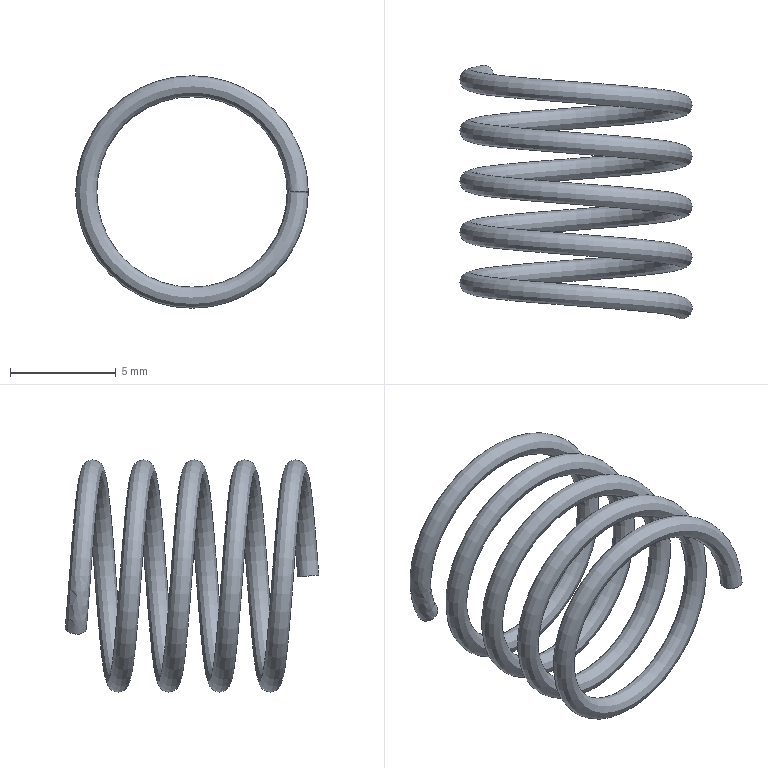Part | NX | features BREP 1 | 1 solid | 3 faces | box 11 x 11.998 x 11 mm | volume 113.166 mm3 | plane 2 | spline 1
STEP:
#1=CARTESIAN_POINT('',(5.,-0.4985,0.03809));
#2=VERTEX_POINT('',#1);
#3=CARTESIAN_POINT('',(5.,0.,0.));
#4=DIRECTION('',(0.,0.07617,0.9971));
#5=DIRECTION('',(0.,-0.9971,0.07617));
#6=AXIS2_PLACEMENT_3D('',#3,#4,#5);
#7=CIRCLE('',#6,0.5);
#8=EDGE_CURVE('',#2,#2,#7,.T.);
#9=ORIENTED_EDGE('',*,*,#8,.F.);
#10=EDGE_LOOP('',(#9));
#11=FACE_BOUND('',#10,.T.);
#12=CARTESIAN_POINT('',(5.,0.4985,-0.03809));
#13=DIRECTION('',(0.,-0.07617,-0.9971));
#14=DIRECTION('',(0.,-0.9971,0.07617));
#15=AXIS2_PLACEMENT_3D('',#12,#13,#14);
#16=PLANE('',#15);
#17=ADVANCED_FACE('',(#11),#16,.T.);
#18=CARTESIAN_POINT('',(-4.311,10.502,-2.533));
#19=VERTEX_POINT('',#18);
#20=CARTESIAN_POINT('',(-4.33,11.001,-2.5));
#21=DIRECTION('',(-0.4985,-0.07617,0.8635));
#22=DIRECTION('',(0.866,0.,0.5));
#23=AXIS2_PLACEMENT_3D('',#20,#21,#22);
#24=CIRCLE('',#23,0.5);
#25=EDGE_CURVE('',#19,#19,#24,.T.);
#26=ORIENTED_EDGE('',*,*,#25,.F.);
#27=EDGE_LOOP('',(#26));
#28=FACE_BOUND('',#27,.T.);
#29=CARTESIAN_POINT('',(-4.349,11.499,-2.467));
#30=DIRECTION('',(-0.4985,-0.07617,0.8635));
#31=DIRECTION('',(-0.866,0.,-0.5));
#32=AXIS2_PLACEMENT_3D('',#29,#30,#31);
#33=PLANE('',#32);
#34=ADVANCED_FACE('',(#28),#33,.F.);
#35=ORIENTED_EDGE('',*,*,#8,.T.);
#36=EDGE_LOOP('',(#35));
#37=FACE_BOUND('',#36,.T.);
#38=ORIENTED_EDGE('',*,*,#25,.T.);
#39=EDGE_LOOP('',(#38));
#40=FACE_BOUND('',#39,.T.);
#41=CARTESIAN_POINT('',(5.,-0.4985,0.03809));
#42=CARTESIAN_POINT('',(4.988,-0.3785,1.663));
#43=CARTESIAN_POINT('',(4.023,-0.2585,2.97));
#44=CARTESIAN_POINT('',(3.058,-0.1385,4.277));
#45=CARTESIAN_POINT('',(1.509,-0.01855,4.767));
#46=CARTESIAN_POINT('',(-0.04005,0.1015,5.257));
#47=CARTESIAN_POINT('',(-1.581,0.2215,4.744));
#48=CARTESIAN_POINT('',(-3.123,0.3415,4.23));
#49=CARTESIAN_POINT('',(-4.067,0.4615,2.908));
#50=CARTESIAN_POINT('',(-5.012,0.5815,1.587));
#51=CARTESIAN_POINT('',(-5.,0.7015,-0.03809));
#52=CARTESIAN_POINT('',(-4.988,0.8215,-1.663));
#53=CARTESIAN_POINT('',(-4.023,0.9415,-2.97));
#54=CARTESIAN_POINT('',(-3.058,1.061,-4.277));
#55=CARTESIAN_POINT('',(-1.509,1.181,-4.767));
#56=CARTESIAN_POINT('',(0.04005,1.301,-5.257));
#57=CARTESIAN_POINT('',(1.581,1.421,-4.744));
#58=CARTESIAN_POINT('',(3.123,1.541,-4.23));
#59=CARTESIAN_POINT('',(4.067,1.661,-2.908));
#60=CARTESIAN_POINT('',(5.012,1.781,-1.587));
#61=CARTESIAN_POINT('',(5.,1.901,0.03809));
#62=CARTESIAN_POINT('',(4.988,2.021,1.663));
#63=CARTESIAN_POINT('',(4.023,2.141,2.97));
#64=CARTESIAN_POINT('',(3.058,2.261,4.277));
#65=CARTESIAN_POINT('',(1.509,2.381,4.767));
#66=CARTESIAN_POINT('',(-0.04005,2.501,5.257));
#67=CARTESIAN_POINT('',(-1.581,2.621,4.744));
#68=CARTESIAN_POINT('',(-3.123,2.741,4.23));
#69=CARTESIAN_POINT('',(-4.067,2.861,2.908));
#70=CARTESIAN_POINT('',(-5.012,2.981,1.587));
#71=CARTESIAN_POINT('',(-5.,3.101,-0.03809));
#72=CARTESIAN_POINT('',(-4.988,3.221,-1.663));
#73=CARTESIAN_POINT('',(-4.023,3.341,-2.97));
#74=CARTESIAN_POINT('',(-3.058,3.461,-4.277));
#75=CARTESIAN_POINT('',(-1.509,3.581,-4.767));
#76=CARTESIAN_POINT('',(0.04005,3.701,-5.257));
#77=CARTESIAN_POINT('',(1.581,3.821,-4.744));
#78=CARTESIAN_POINT('',(3.123,3.941,-4.23));
#79=CARTESIAN_POINT('',(4.067,4.061,-2.908));
#80=CARTESIAN_POINT('',(5.012,4.181,-1.587));
#81=CARTESIAN_POINT('',(5.,4.301,0.03809));
#82=CARTESIAN_POINT('',(4.988,4.421,1.663));
#83=CARTESIAN_POINT('',(4.023,4.541,2.97));
#84=CARTESIAN_POINT('',(3.058,4.661,4.277));
#85=CARTESIAN_POINT('',(1.509,4.781,4.767));
#86=CARTESIAN_POINT('',(-0.04005,4.901,5.257));
#87=CARTESIAN_POINT('',(-1.581,5.021,4.744));
#88=CARTESIAN_POINT('',(-3.123,5.141,4.23));
#89=CARTESIAN_POINT('',(-4.067,5.261,2.908));
#90=CARTESIAN_POINT('',(-5.012,5.381,1.587));
#91=CARTESIAN_POINT('',(-5.,5.501,-0.03809));
#92=CARTESIAN_POINT('',(-4.988,5.621,-1.663));
#93=CARTESIAN_POINT('',(-4.023,5.741,-2.97));
#94=CARTESIAN_POINT('',(-3.058,5.861,-4.277));
#95=CARTESIAN_POINT('',(-1.509,5.981,-4.767));
#96=CARTESIAN_POINT('',(0.04005,6.101,-5.257));
#97=CARTESIAN_POINT('',(1.581,6.221,-4.744));
#98=CARTESIAN_POINT('',(3.123,6.341,-4.23));
#99=CARTESIAN_POINT('',(4.067,6.461,-2.908));
#100=CARTESIAN_POINT('',(5.012,6.581,-1.587));
#101=CARTESIAN_POINT('',(5.,6.701,0.03809));
#102=CARTESIAN_POINT('',(4.988,6.821,1.663));
#103=CARTESIAN_POINT('',(4.023,6.941,2.97));
#104=CARTESIAN_POINT('',(3.058,7.061,4.277));
#105=CARTESIAN_POINT('',(1.509,7.181,4.767));
#106=CARTESIAN_POINT('',(-0.04005,7.301,5.257));
#107=CARTESIAN_POINT('',(-1.581,7.421,4.744));
#108=CARTESIAN_POINT('',(-3.123,7.541,4.23));
#109=CARTESIAN_POINT('',(-4.067,7.661,2.908));
#110=CARTESIAN_POINT('',(-5.012,7.781,1.587));
#111=CARTESIAN_POINT('',(-5.,7.901,-0.03809));
#112=CARTESIAN_POINT('',(-4.988,8.021,-1.663));
#113=CARTESIAN_POINT('',(-4.023,8.141,-2.97));
#114=CARTESIAN_POINT('',(-3.058,8.261,-4.277));
#115=CARTESIAN_POINT('',(-1.509,8.381,-4.767));
#116=CARTESIAN_POINT('',(0.04005,8.501,-5.257));
#117=CARTESIAN_POINT('',(1.581,8.621,-4.744));
#118=CARTESIAN_POINT('',(3.123,8.741,-4.23));
#119=CARTESIAN_POINT('',(4.067,8.861,-2.908));
#120=CARTESIAN_POINT('',(5.012,8.981,-1.587));
#121=CARTESIAN_POINT('',(5.,9.101,0.03809));
#122=CARTESIAN_POINT('',(4.988,9.221,1.663));
#123=CARTESIAN_POINT('',(4.023,9.341,2.97));
#124=CARTESIAN_POINT('',(3.058,9.461,4.277));
#125=CARTESIAN_POINT('',(1.509,9.581,4.767));
#126=CARTESIAN_POINT('',(-0.04005,9.701,5.257));
#127=CARTESIAN_POINT('',(-1.581,9.821,4.744));
#128=CARTESIAN_POINT('',(-3.123,9.941,4.23));
#129=CARTESIAN_POINT('',(-4.067,10.061,2.908));
#130=CARTESIAN_POINT('',(-5.012,10.181,1.587));
#131=CARTESIAN_POINT('',(-5.,10.301,-0.03809));
#132=CARTESIAN_POINT('',(-4.99,10.4,-1.378));
#133=CARTESIAN_POINT('',(-4.311,10.502,-2.533));
#134=CARTESIAN_POINT('',(6.,-0.4985,0.03809));
#135=CARTESIAN_POINT('',(5.988,-0.3785,1.988));
#136=CARTESIAN_POINT('',(4.832,-0.2585,3.558));
#137=CARTESIAN_POINT('',(3.676,-0.1385,5.127));
#138=CARTESIAN_POINT('',(1.818,-0.01855,5.718));
#139=CARTESIAN_POINT('',(-0.04005,0.1015,6.309));
#140=CARTESIAN_POINT('',(-1.89,0.2215,5.695));
#141=CARTESIAN_POINT('',(-3.741,0.3415,5.08));
#142=CARTESIAN_POINT('',(-4.876,0.4615,3.496));
#143=CARTESIAN_POINT('',(-6.012,0.5815,1.911));
#144=CARTESIAN_POINT('',(-6.,0.7015,-0.03809));
#145=CARTESIAN_POINT('',(-5.988,0.8215,-1.988));
#146=CARTESIAN_POINT('',(-4.832,0.9415,-3.558));
#147=CARTESIAN_POINT('',(-3.676,1.061,-5.127));
#148=CARTESIAN_POINT('',(-1.818,1.181,-5.718));
#149=CARTESIAN_POINT('',(0.04005,1.301,-6.309));
#150=CARTESIAN_POINT('',(1.89,1.421,-5.695));
#151=CARTESIAN_POINT('',(3.741,1.541,-5.08));
#152=CARTESIAN_POINT('',(4.876,1.661,-3.496));
#153=CARTESIAN_POINT('',(6.012,1.781,-1.911));
#154=CARTESIAN_POINT('',(6.,1.901,0.03809));
#155=CARTESIAN_POINT('',(5.988,2.021,1.988));
#156=CARTESIAN_POINT('',(4.832,2.141,3.558));
#157=CARTESIAN_POINT('',(3.676,2.261,5.127));
#158=CARTESIAN_POINT('',(1.818,2.381,5.718));
#159=CARTESIAN_POINT('',(-0.04005,2.501,6.309));
#160=CARTESIAN_POINT('',(-1.89,2.621,5.695));
#161=CARTESIAN_POINT('',(-3.741,2.741,5.08));
#162=CARTESIAN_POINT('',(-4.876,2.861,3.496));
#163=CARTESIAN_POINT('',(-6.012,2.981,1.911));
#164=CARTESIAN_POINT('',(-6.,3.101,-0.03809));
#165=CARTESIAN_POINT('',(-5.988,3.221,-1.988));
#166=CARTESIAN_POINT('',(-4.832,3.341,-3.558));
#167=CARTESIAN_POINT('',(-3.676,3.461,-5.127));
#168=CARTESIAN_POINT('',(-1.818,3.581,-5.718));
#169=CARTESIAN_POINT('',(0.04005,3.701,-6.309));
#170=CARTESIAN_POINT('',(1.89,3.821,-5.695));
#171=CARTESIAN_POINT('',(3.741,3.941,-5.08));
#172=CARTESIAN_POINT('',(4.876,4.061,-3.496));
#173=CARTESIAN_POINT('',(6.012,4.181,-1.911));
#174=CARTESIAN_POINT('',(6.,4.301,0.03809));
#175=CARTESIAN_POINT('',(5.988,4.421,1.988));
#176=CARTESIAN_POINT('',(4.832,4.541,3.558));
#177=CARTESIAN_POINT('',(3.676,4.661,5.127));
#178=CARTESIAN_POINT('',(1.818,4.781,5.718));
#179=CARTESIAN_POINT('',(-0.04005,4.901,6.309));
#180=CARTESIAN_POINT('',(-1.89,5.021,5.695));
#181=CARTESIAN_POINT('',(-3.741,5.141,5.08));
#182=CARTESIAN_POINT('',(-4.876,5.261,3.496));
#183=CARTESIAN_POINT('',(-6.012,5.381,1.911));
#184=CARTESIAN_POINT('',(-6.,5.501,-0.03809));
#185=CARTESIAN_POINT('',(-5.988,5.621,-1.988));
#186=CARTESIAN_POINT('',(-4.832,5.741,-3.558));
#187=CARTESIAN_POINT('',(-3.676,5.861,-5.127));
#188=CARTESIAN_POINT('',(-1.818,5.981,-5.718));
#189=CARTESIAN_POINT('',(0.04005,6.101,-6.309));
#190=CARTESIAN_POINT('',(1.89,6.221,-5.695));
#191=CARTESIAN_POINT('',(3.741,6.341,-5.08));
#192=CARTESIAN_POINT('',(4.876,6.461,-3.496));
#193=CARTESIAN_POINT('',(6.012,6.581,-1.911));
#194=CARTESIAN_POINT('',(6.,6.701,0.03809));
#195=CARTESIAN_POINT('',(5.988,6.821,1.988));
#196=CARTESIAN_POINT('',(4.832,6.941,3.558));
#197=CARTESIAN_POINT('',(3.676,7.061,5.127));
#198=CARTESIAN_POINT('',(1.818,7.181,5.718));
#199=CARTESIAN_POINT('',(-0.04005,7.301,6.309));
#200=CARTESIAN_POINT('',(-1.89,7.421,5.695));
#201=CARTESIAN_POINT('',(-3.741,7.541,5.08));
#202=CARTESIAN_POINT('',(-4.876,7.661,3.496));
#203=CARTESIAN_POINT('',(-6.012,7.781,1.911));
#204=CARTESIAN_POINT('',(-6.,7.901,-0.03809));
#205=CARTESIAN_POINT('',(-5.988,8.021,-1.988));
#206=CARTESIAN_POINT('',(-4.832,8.141,-3.558));
#207=CARTESIAN_POINT('',(-3.676,8.261,-5.127));
#208=CARTESIAN_POINT('',(-1.818,8.381,-5.718));
#209=CARTESIAN_POINT('',(0.04005,8.501,-6.309));
#210=CARTESIAN_POINT('',(1.89,8.621,-5.695));
#211=CARTESIAN_POINT('',(3.741,8.741,-5.08));
#212=CARTESIAN_POINT('',(4.876,8.861,-3.496));
#213=CARTESIAN_POINT('',(6.012,8.981,-1.911));
#214=CARTESIAN_POINT('',(6.,9.101,0.03809));
#215=CARTESIAN_POINT('',(5.988,9.221,1.988));
#216=CARTESIAN_POINT('',(4.832,9.341,3.558));
#217=CARTESIAN_POINT('',(3.676,9.461,5.127));
#218=CARTESIAN_POINT('',(1.818,9.581,5.718));
#219=CARTESIAN_POINT('',(-0.04005,9.701,6.309));
#220=CARTESIAN_POINT('',(-1.89,9.821,5.695));
#221=CARTESIAN_POINT('',(-3.741,9.941,5.08));
#222=CARTESIAN_POINT('',(-4.876,10.061,3.496));
#223=CARTESIAN_POINT('',(-6.012,10.181,1.911));
#224=CARTESIAN_POINT('',(-6.,10.301,-0.03809));
#225=CARTESIAN_POINT('',(-5.99,10.4,-1.646));
#226=CARTESIAN_POINT('',(-5.177,10.502,-3.033));
#227=CARTESIAN_POINT('',(6.,0.4985,-0.03809));
#228=CARTESIAN_POINT('',(6.012,0.6185,1.911));
#229=CARTESIAN_POINT('',(4.876,0.7385,3.496));
#230=CARTESIAN_POINT('',(3.741,0.8585,5.08));
#231=CARTESIAN_POINT('',(1.89,0.9785,5.695));
#232=CARTESIAN_POINT('',(0.04005,1.099,6.309));
#233=CARTESIAN_POINT('',(-1.818,1.219,5.718));
#234=CARTESIAN_POINT('',(-3.676,1.339,5.127));
#235=CARTESIAN_POINT('',(-4.832,1.459,3.558));
#236=CARTESIAN_POINT('',(-5.988,1.579,1.988));
#237=CARTESIAN_POINT('',(-6.,1.699,0.03809));
#238=CARTESIAN_POINT('',(-6.012,1.819,-1.911));
#239=CARTESIAN_POINT('',(-4.876,1.939,-3.496));
#240=CARTESIAN_POINT('',(-3.741,2.059,-5.08));
#241=CARTESIAN_POINT('',(-1.89,2.179,-5.695));
#242=CARTESIAN_POINT('',(-0.04005,2.299,-6.309));
#243=CARTESIAN_POINT('',(1.818,2.419,-5.718));
#244=CARTESIAN_POINT('',(3.676,2.539,-5.127));
#245=CARTESIAN_POINT('',(4.832,2.659,-3.558));
#246=CARTESIAN_POINT('',(5.988,2.779,-1.988));
#247=CARTESIAN_POINT('',(6.,2.899,-0.03809));
#248=CARTESIAN_POINT('',(6.012,3.019,1.911));
#249=CARTESIAN_POINT('',(4.876,3.139,3.496));
#250=CARTESIAN_POINT('',(3.741,3.259,5.08));
#251=CARTESIAN_POINT('',(1.89,3.379,5.695));
#252=CARTESIAN_POINT('',(0.04005,3.499,6.309));
#253=CARTESIAN_POINT('',(-1.818,3.619,5.718));
#254=CARTESIAN_POINT('',(-3.676,3.739,5.127));
#255=CARTESIAN_POINT('',(-4.832,3.859,3.558));
#256=CARTESIAN_POINT('',(-5.988,3.979,1.988));
#257=CARTESIAN_POINT('',(-6.,4.099,0.03809));
#258=CARTESIAN_POINT('',(-6.012,4.219,-1.911));
#259=CARTESIAN_POINT('',(-4.876,4.339,-3.496));
#260=CARTESIAN_POINT('',(-3.741,4.459,-5.08));
#261=CARTESIAN_POINT('',(-1.89,4.579,-5.695));
#262=CARTESIAN_POINT('',(-0.04005,4.699,-6.309));
#263=CARTESIAN_POINT('',(1.818,4.819,-5.718));
#264=CARTESIAN_POINT('',(3.676,4.939,-5.127));
#265=CARTESIAN_POINT('',(4.832,5.059,-3.558));
#266=CARTESIAN_POINT('',(5.988,5.179,-1.988));
#267=CARTESIAN_POINT('',(6.,5.299,-0.03809));
#268=CARTESIAN_POINT('',(6.012,5.419,1.911));
#269=CARTESIAN_POINT('',(4.876,5.539,3.496));
#270=CARTESIAN_POINT('',(3.741,5.659,5.08));
#271=CARTESIAN_POINT('',(1.89,5.779,5.695));
#272=CARTESIAN_POINT('',(0.04005,5.899,6.309));
#273=CARTESIAN_POINT('',(-1.818,6.019,5.718));
#274=CARTESIAN_POINT('',(-3.676,6.139,5.127));
#275=CARTESIAN_POINT('',(-4.832,6.259,3.558));
#276=CARTESIAN_POINT('',(-5.988,6.379,1.988));
#277=CARTESIAN_POINT('',(-6.,6.499,0.03809));
#278=CARTESIAN_POINT('',(-6.012,6.619,-1.911));
#279=CARTESIAN_POINT('',(-4.876,6.739,-3.496));
#280=CARTESIAN_POINT('',(-3.741,6.859,-5.08));
#281=CARTESIAN_POINT('',(-1.89,6.979,-5.695));
#282=CARTESIAN_POINT('',(-0.04005,7.099,-6.309));
#283=CARTESIAN_POINT('',(1.818,7.219,-5.718));
#284=CARTESIAN_POINT('',(3.676,7.339,-5.127));
#285=CARTESIAN_POINT('',(4.832,7.459,-3.558));
#286=CARTESIAN_POINT('',(5.988,7.579,-1.988));
#287=CARTESIAN_POINT('',(6.,7.699,-0.03809));
#288=CARTESIAN_POINT('',(6.012,7.819,1.911));
#289=CARTESIAN_POINT('',(4.876,7.939,3.496));
#290=CARTESIAN_POINT('',(3.741,8.059,5.08));
#291=CARTESIAN_POINT('',(1.89,8.179,5.695));
#292=CARTESIAN_POINT('',(0.04005,8.299,6.309));
#293=CARTESIAN_POINT('',(-1.818,8.419,5.718));
#294=CARTESIAN_POINT('',(-3.676,8.539,5.127));
#295=CARTESIAN_POINT('',(-4.832,8.659,3.558));
#296=CARTESIAN_POINT('',(-5.988,8.779,1.988));
#297=CARTESIAN_POINT('',(-6.,8.899,0.03809));
#298=CARTESIAN_POINT('',(-6.012,9.019,-1.911));
#299=CARTESIAN_POINT('',(-4.876,9.139,-3.496));
#300=CARTESIAN_POINT('',(-3.741,9.259,-5.08));
#301=CARTESIAN_POINT('',(-1.89,9.379,-5.695));
#302=CARTESIAN_POINT('',(-0.04005,9.499,-6.309));
#303=CARTESIAN_POINT('',(1.818,9.619,-5.718));
#304=CARTESIAN_POINT('',(3.676,9.739,-5.127));
#305=CARTESIAN_POINT('',(4.832,9.859,-3.558));
#306=CARTESIAN_POINT('',(5.988,9.979,-1.988));
#307=CARTESIAN_POINT('',(6.,10.099,-0.03809));
#308=CARTESIAN_POINT('',(6.012,10.219,1.911));
#309=CARTESIAN_POINT('',(4.876,10.339,3.496));
#310=CARTESIAN_POINT('',(3.741,10.459,5.08));
#311=CARTESIAN_POINT('',(1.89,10.579,5.695));
#312=CARTESIAN_POINT('',(0.04005,10.699,6.309));
#313=CARTESIAN_POINT('',(-1.818,10.819,5.718));
#314=CARTESIAN_POINT('',(-3.676,10.939,5.127));
#315=CARTESIAN_POINT('',(-4.832,11.059,3.558));
#316=CARTESIAN_POINT('',(-5.988,11.179,1.988));
#317=CARTESIAN_POINT('',(-6.,11.299,0.03809));
#318=CARTESIAN_POINT('',(-6.01,11.398,-1.57));
#319=CARTESIAN_POINT('',(-5.215,11.499,-2.967));
#320=CARTESIAN_POINT('',(5.,0.4985,-0.03809));
#321=CARTESIAN_POINT('',(5.012,0.6185,1.587));
#322=CARTESIAN_POINT('',(4.067,0.7385,2.908));
#323=CARTESIAN_POINT('',(3.123,0.8585,4.23));
#324=CARTESIAN_POINT('',(1.581,0.9785,4.744));
#325=CARTESIAN_POINT('',(0.04005,1.099,5.257));
#326=CARTESIAN_POINT('',(-1.509,1.219,4.767));
#327=CARTESIAN_POINT('',(-3.058,1.339,4.277));
#328=CARTESIAN_POINT('',(-4.023,1.459,2.97));
#329=CARTESIAN_POINT('',(-4.988,1.579,1.663));
#330=CARTESIAN_POINT('',(-5.,1.699,0.03809));
#331=CARTESIAN_POINT('',(-5.012,1.819,-1.587));
#332=CARTESIAN_POINT('',(-4.067,1.939,-2.908));
#333=CARTESIAN_POINT('',(-3.123,2.059,-4.23));
#334=CARTESIAN_POINT('',(-1.581,2.179,-4.744));
#335=CARTESIAN_POINT('',(-0.04005,2.299,-5.257));
#336=CARTESIAN_POINT('',(1.509,2.419,-4.767));
#337=CARTESIAN_POINT('',(3.058,2.539,-4.277));
#338=CARTESIAN_POINT('',(4.023,2.659,-2.97));
#339=CARTESIAN_POINT('',(4.988,2.779,-1.663));
#340=CARTESIAN_POINT('',(5.,2.899,-0.03809));
#341=CARTESIAN_POINT('',(5.012,3.019,1.587));
#342=CARTESIAN_POINT('',(4.067,3.139,2.908));
#343=CARTESIAN_POINT('',(3.123,3.259,4.23));
#344=CARTESIAN_POINT('',(1.581,3.379,4.744));
#345=CARTESIAN_POINT('',(0.04005,3.499,5.257));
#346=CARTESIAN_POINT('',(-1.509,3.619,4.767));
#347=CARTESIAN_POINT('',(-3.058,3.739,4.277));
#348=CARTESIAN_POINT('',(-4.023,3.859,2.97));
#349=CARTESIAN_POINT('',(-4.988,3.979,1.663));
#350=CARTESIAN_POINT('',(-5.,4.099,0.03809));
#351=CARTESIAN_POINT('',(-5.012,4.219,-1.587));
#352=CARTESIAN_POINT('',(-4.067,4.339,-2.908));
#353=CARTESIAN_POINT('',(-3.123,4.459,-4.23));
#354=CARTESIAN_POINT('',(-1.581,4.579,-4.744));
#355=CARTESIAN_POINT('',(-0.04005,4.699,-5.257));
#356=CARTESIAN_POINT('',(1.509,4.819,-4.767));
#357=CARTESIAN_POINT('',(3.058,4.939,-4.277));
#358=CARTESIAN_POINT('',(4.023,5.059,-2.97));
#359=CARTESIAN_POINT('',(4.988,5.179,-1.663));
#360=CARTESIAN_POINT('',(5.,5.299,-0.03809));
#361=CARTESIAN_POINT('',(5.012,5.419,1.587));
#362=CARTESIAN_POINT('',(4.067,5.539,2.908));
#363=CARTESIAN_POINT('',(3.123,5.659,4.23));
#364=CARTESIAN_POINT('',(1.581,5.779,4.744));
#365=CARTESIAN_POINT('',(0.04005,5.899,5.257));
#366=CARTESIAN_POINT('',(-1.509,6.019,4.767));
#367=CARTESIAN_POINT('',(-3.058,6.139,4.277));
#368=CARTESIAN_POINT('',(-4.023,6.259,2.97));
#369=CARTESIAN_POINT('',(-4.988,6.379,1.663));
#370=CARTESIAN_POINT('',(-5.,6.499,0.03809));
#371=CARTESIAN_POINT('',(-5.012,6.619,-1.587));
#372=CARTESIAN_POINT('',(-4.067,6.739,-2.908));
#373=CARTESIAN_POINT('',(-3.123,6.859,-4.23));
#374=CARTESIAN_POINT('',(-1.581,6.979,-4.744));
#375=CARTESIAN_POINT('',(-0.04005,7.099,-5.257));
#376=CARTESIAN_POINT('',(1.509,7.219,-4.767));
#377=CARTESIAN_POINT('',(3.058,7.339,-4.277));
#378=CARTESIAN_POINT('',(4.023,7.459,-2.97));
#379=CARTESIAN_POINT('',(4.988,7.579,-1.663));
#380=CARTESIAN_POINT('',(5.,7.699,-0.03809));
#381=CARTESIAN_POINT('',(5.012,7.819,1.587));
#382=CARTESIAN_POINT('',(4.067,7.939,2.908));
#383=CARTESIAN_POINT('',(3.123,8.059,4.23));
#384=CARTESIAN_POINT('',(1.581,8.179,4.744));
#385=CARTESIAN_POINT('',(0.04005,8.299,5.257));
#386=CARTESIAN_POINT('',(-1.509,8.419,4.767));
#387=CARTESIAN_POINT('',(-3.058,8.539,4.277));
#388=CARTESIAN_POINT('',(-4.023,8.659,2.97));
#389=CARTESIAN_POINT('',(-4.988,8.779,1.663));
#390=CARTESIAN_POINT('',(-5.,8.899,0.03809));
#391=CARTESIAN_POINT('',(-5.012,9.019,-1.587));
#392=CARTESIAN_POINT('',(-4.067,9.139,-2.908));
#393=CARTESIAN_POINT('',(-3.123,9.259,-4.23));
#394=CARTESIAN_POINT('',(-1.581,9.379,-4.744));
#395=CARTESIAN_POINT('',(-0.04005,9.499,-5.257));
#396=CARTESIAN_POINT('',(1.509,9.619,-4.767));
#397=CARTESIAN_POINT('',(3.058,9.739,-4.277));
#398=CARTESIAN_POINT('',(4.023,9.859,-2.97));
#399=CARTESIAN_POINT('',(4.988,9.979,-1.663));
#400=CARTESIAN_POINT('',(5.,10.099,-0.03809));
#401=CARTESIAN_POINT('',(5.012,10.219,1.587));
#402=CARTESIAN_POINT('',(4.067,10.339,2.908));
#403=CARTESIAN_POINT('',(3.123,10.459,4.23));
#404=CARTESIAN_POINT('',(1.581,10.579,4.744));
#405=CARTESIAN_POINT('',(0.04005,10.699,5.257));
#406=CARTESIAN_POINT('',(-1.509,10.819,4.767));
#407=CARTESIAN_POINT('',(-3.058,10.939,4.277));
#408=CARTESIAN_POINT('',(-4.023,11.059,2.97));
#409=CARTESIAN_POINT('',(-4.988,11.179,1.663));
#410=CARTESIAN_POINT('',(-5.,11.299,0.03809));
#411=CARTESIAN_POINT('',(-5.01,11.398,-1.302));
#412=CARTESIAN_POINT('',(-4.349,11.499,-2.467));
#413=CARTESIAN_POINT('',(4.,0.4985,-0.03809));
#414=CARTESIAN_POINT('',(4.012,0.6185,1.262));
#415=CARTESIAN_POINT('',(3.258,0.7385,2.32));
#416=CARTESIAN_POINT('',(2.505,0.8585,3.379));
#417=CARTESIAN_POINT('',(1.272,0.9785,3.792));
#418=CARTESIAN_POINT('',(0.04005,1.099,4.206));
#419=CARTESIAN_POINT('',(-1.2,1.219,3.816));
#420=CARTESIAN_POINT('',(-2.44,1.339,3.426));
#421=CARTESIAN_POINT('',(-3.214,1.459,2.382));
#422=CARTESIAN_POINT('',(-3.988,1.579,1.338));
#423=CARTESIAN_POINT('',(-4.,1.699,0.03809));
#424=CARTESIAN_POINT('',(-4.012,1.819,-1.262));
#425=CARTESIAN_POINT('',(-3.258,1.939,-2.32));
#426=CARTESIAN_POINT('',(-2.505,2.059,-3.379));
#427=CARTESIAN_POINT('',(-1.272,2.179,-3.792));
#428=CARTESIAN_POINT('',(-0.04005,2.299,-4.206));
#429=CARTESIAN_POINT('',(1.2,2.419,-3.816));
#430=CARTESIAN_POINT('',(2.44,2.539,-3.426));
#431=CARTESIAN_POINT('',(3.214,2.659,-2.382));
#432=CARTESIAN_POINT('',(3.988,2.779,-1.338));
#433=CARTESIAN_POINT('',(4.,2.899,-0.03809));
#434=CARTESIAN_POINT('',(4.012,3.019,1.262));
#435=CARTESIAN_POINT('',(3.258,3.139,2.32));
#436=CARTESIAN_POINT('',(2.505,3.259,3.379));
#437=CARTESIAN_POINT('',(1.272,3.379,3.792));
#438=CARTESIAN_POINT('',(0.04005,3.499,4.206));
#439=CARTESIAN_POINT('',(-1.2,3.619,3.816));
#440=CARTESIAN_POINT('',(-2.44,3.739,3.426));
#441=CARTESIAN_POINT('',(-3.214,3.859,2.382));
#442=CARTESIAN_POINT('',(-3.988,3.979,1.338));
#443=CARTESIAN_POINT('',(-4.,4.099,0.03809));
#444=CARTESIAN_POINT('',(-4.012,4.219,-1.262));
#445=CARTESIAN_POINT('',(-3.258,4.339,-2.32));
#446=CARTESIAN_POINT('',(-2.505,4.459,-3.379));
#447=CARTESIAN_POINT('',(-1.272,4.579,-3.792));
#448=CARTESIAN_POINT('',(-0.04005,4.699,-4.206));
#449=CARTESIAN_POINT('',(1.2,4.819,-3.816));
#450=CARTESIAN_POINT('',(2.44,4.939,-3.426));
#451=CARTESIAN_POINT('',(3.214,5.059,-2.382));
#452=CARTESIAN_POINT('',(3.988,5.179,-1.338));
#453=CARTESIAN_POINT('',(4.,5.299,-0.03809));
#454=CARTESIAN_POINT('',(4.012,5.419,1.262));
#455=CARTESIAN_POINT('',(3.258,5.539,2.32));
#456=CARTESIAN_POINT('',(2.505,5.659,3.379));
#457=CARTESIAN_POINT('',(1.272,5.779,3.792));
#458=CARTESIAN_POINT('',(0.04005,5.899,4.206));
#459=CARTESIAN_POINT('',(-1.2,6.019,3.816));
#460=CARTESIAN_POINT('',(-2.44,6.139,3.426));
#461=CARTESIAN_POINT('',(-3.214,6.259,2.382));
#462=CARTESIAN_POINT('',(-3.988,6.379,1.338));
#463=CARTESIAN_POINT('',(-4.,6.499,0.03809));
#464=CARTESIAN_POINT('',(-4.012,6.619,-1.262));
#465=CARTESIAN_POINT('',(-3.258,6.739,-2.32));
#466=CARTESIAN_POINT('',(-2.505,6.859,-3.379));
#467=CARTESIAN_POINT('',(-1.272,6.979,-3.792));
#468=CARTESIAN_POINT('',(-0.04005,7.099,-4.206));
#469=CARTESIAN_POINT('',(1.2,7.219,-3.816));
#470=CARTESIAN_POINT('',(2.44,7.339,-3.426));
#471=CARTESIAN_POINT('',(3.214,7.459,-2.382));
#472=CARTESIAN_POINT('',(3.988,7.579,-1.338));
#473=CARTESIAN_POINT('',(4.,7.699,-0.03809));
#474=CARTESIAN_POINT('',(4.012,7.819,1.262));
#475=CARTESIAN_POINT('',(3.258,7.939,2.32));
#476=CARTESIAN_POINT('',(2.505,8.059,3.379));
#477=CARTESIAN_POINT('',(1.272,8.179,3.792));
#478=CARTESIAN_POINT('',(0.04005,8.299,4.206));
#479=CARTESIAN_POINT('',(-1.2,8.419,3.816));
#480=CARTESIAN_POINT('',(-2.44,8.539,3.426));
#481=CARTESIAN_POINT('',(-3.214,8.659,2.382));
#482=CARTESIAN_POINT('',(-3.988,8.779,1.338));
#483=CARTESIAN_POINT('',(-4.,8.899,0.03809));
#484=CARTESIAN_POINT('',(-4.012,9.019,-1.262));
#485=CARTESIAN_POINT('',(-3.258,9.139,-2.32));
#486=CARTESIAN_POINT('',(-2.505,9.259,-3.379));
#487=CARTESIAN_POINT('',(-1.272,9.379,-3.792));
#488=CARTESIAN_POINT('',(-0.04005,9.499,-4.206));
#489=CARTESIAN_POINT('',(1.2,9.619,-3.816));
#490=CARTESIAN_POINT('',(2.44,9.739,-3.426));
#491=CARTESIAN_POINT('',(3.214,9.859,-2.382));
#492=CARTESIAN_POINT('',(3.988,9.979,-1.338));
#493=CARTESIAN_POINT('',(4.,10.099,-0.03809));
#494=CARTESIAN_POINT('',(4.012,10.219,1.262));
#495=CARTESIAN_POINT('',(3.258,10.339,2.32));
#496=CARTESIAN_POINT('',(2.505,10.459,3.379));
#497=CARTESIAN_POINT('',(1.272,10.579,3.792));
#498=CARTESIAN_POINT('',(0.04005,10.699,4.206));
#499=CARTESIAN_POINT('',(-1.2,10.819,3.816));
#500=CARTESIAN_POINT('',(-2.44,10.939,3.426));
#501=CARTESIAN_POINT('',(-3.214,11.059,2.382));
#502=CARTESIAN_POINT('',(-3.988,11.179,1.338));
#503=CARTESIAN_POINT('',(-4.,11.299,0.03809));
#504=CARTESIAN_POINT('',(-4.01,11.398,-1.034));
#505=CARTESIAN_POINT('',(-3.483,11.499,-1.967));
#506=CARTESIAN_POINT('',(4.,-0.4985,0.03809));
#507=CARTESIAN_POINT('',(3.988,-0.3785,1.338));
#508=CARTESIAN_POINT('',(3.214,-0.2585,2.382));
#509=CARTESIAN_POINT('',(2.44,-0.1385,3.426));
#510=CARTESIAN_POINT('',(1.2,-0.01855,3.816));
#511=CARTESIAN_POINT('',(-0.04005,0.1015,4.206));
#512=CARTESIAN_POINT('',(-1.272,0.2215,3.792));
#513=CARTESIAN_POINT('',(-2.505,0.3415,3.379));
#514=CARTESIAN_POINT('',(-3.258,0.4615,2.32));
#515=CARTESIAN_POINT('',(-4.012,0.5815,1.262));
#516=CARTESIAN_POINT('',(-4.,0.7015,-0.03809));
#517=CARTESIAN_POINT('',(-3.988,0.8215,-1.338));
#518=CARTESIAN_POINT('',(-3.214,0.9415,-2.382));
#519=CARTESIAN_POINT('',(-2.44,1.061,-3.426));
#520=CARTESIAN_POINT('',(-1.2,1.181,-3.816));
#521=CARTESIAN_POINT('',(0.04005,1.301,-4.206));
#522=CARTESIAN_POINT('',(1.272,1.421,-3.792));
#523=CARTESIAN_POINT('',(2.505,1.541,-3.379));
#524=CARTESIAN_POINT('',(3.258,1.661,-2.32));
#525=CARTESIAN_POINT('',(4.012,1.781,-1.262));
#526=CARTESIAN_POINT('',(4.,1.901,0.03809));
#527=CARTESIAN_POINT('',(3.988,2.021,1.338));
#528=CARTESIAN_POINT('',(3.214,2.141,2.382));
#529=CARTESIAN_POINT('',(2.44,2.261,3.426));
#530=CARTESIAN_POINT('',(1.2,2.381,3.816));
#531=CARTESIAN_POINT('',(-0.04005,2.501,4.206));
#532=CARTESIAN_POINT('',(-1.272,2.621,3.792));
#533=CARTESIAN_POINT('',(-2.505,2.741,3.379));
#534=CARTESIAN_POINT('',(-3.258,2.861,2.32));
#535=CARTESIAN_POINT('',(-4.012,2.981,1.262));
#536=CARTESIAN_POINT('',(-4.,3.101,-0.03809));
#537=CARTESIAN_POINT('',(-3.988,3.221,-1.338));
#538=CARTESIAN_POINT('',(-3.214,3.341,-2.382));
#539=CARTESIAN_POINT('',(-2.44,3.461,-3.426));
#540=CARTESIAN_POINT('',(-1.2,3.581,-3.816));
#541=CARTESIAN_POINT('',(0.04005,3.701,-4.206));
#542=CARTESIAN_POINT('',(1.272,3.821,-3.792));
#543=CARTESIAN_POINT('',(2.505,3.941,-3.379));
#544=CARTESIAN_POINT('',(3.258,4.061,-2.32));
#545=CARTESIAN_POINT('',(4.012,4.181,-1.262));
#546=CARTESIAN_POINT('',(4.,4.301,0.03809));
#547=CARTESIAN_POINT('',(3.988,4.421,1.338));
#548=CARTESIAN_POINT('',(3.214,4.541,2.382));
#549=CARTESIAN_POINT('',(2.44,4.661,3.426));
#550=CARTESIAN_POINT('',(1.2,4.781,3.816));
#551=CARTESIAN_POINT('',(-0.04005,4.901,4.206));
#552=CARTESIAN_POINT('',(-1.272,5.021,3.792));
#553=CARTESIAN_POINT('',(-2.505,5.141,3.379));
#554=CARTESIAN_POINT('',(-3.258,5.261,2.32));
#555=CARTESIAN_POINT('',(-4.012,5.381,1.262));
#556=CARTESIAN_POINT('',(-4.,5.501,-0.03809));
#557=CARTESIAN_POINT('',(-3.988,5.621,-1.338));
#558=CARTESIAN_POINT('',(-3.214,5.741,-2.382));
#559=CARTESIAN_POINT('',(-2.44,5.861,-3.426));
#560=CARTESIAN_POINT('',(-1.2,5.981,-3.816));
#561=CARTESIAN_POINT('',(0.04005,6.101,-4.206));
#562=CARTESIAN_POINT('',(1.272,6.221,-3.792));
#563=CARTESIAN_POINT('',(2.505,6.341,-3.379));
#564=CARTESIAN_POINT('',(3.258,6.461,-2.32));
#565=CARTESIAN_POINT('',(4.012,6.581,-1.262));
#566=CARTESIAN_POINT('',(4.,6.701,0.03809));
#567=CARTESIAN_POINT('',(3.988,6.821,1.338));
#568=CARTESIAN_POINT('',(3.214,6.941,2.382));
#569=CARTESIAN_POINT('',(2.44,7.061,3.426));
#570=CARTESIAN_POINT('',(1.2,7.181,3.816));
#571=CARTESIAN_POINT('',(-0.04005,7.301,4.206));
#572=CARTESIAN_POINT('',(-1.272,7.421,3.792));
#573=CARTESIAN_POINT('',(-2.505,7.541,3.379));
#574=CARTESIAN_POINT('',(-3.258,7.661,2.32));
#575=CARTESIAN_POINT('',(-4.012,7.781,1.262));
#576=CARTESIAN_POINT('',(-4.,7.901,-0.03809));
#577=CARTESIAN_POINT('',(-3.988,8.021,-1.338));
#578=CARTESIAN_POINT('',(-3.214,8.141,-2.382));
#579=CARTESIAN_POINT('',(-2.44,8.261,-3.426));
#580=CARTESIAN_POINT('',(-1.2,8.381,-3.816));
#581=CARTESIAN_POINT('',(0.04005,8.501,-4.206));
#582=CARTESIAN_POINT('',(1.272,8.621,-3.792));
#583=CARTESIAN_POINT('',(2.505,8.741,-3.379));
#584=CARTESIAN_POINT('',(3.258,8.861,-2.32));
#585=CARTESIAN_POINT('',(4.012,8.981,-1.262));
#586=CARTESIAN_POINT('',(4.,9.101,0.03809));
#587=CARTESIAN_POINT('',(3.988,9.221,1.338));
#588=CARTESIAN_POINT('',(3.214,9.341,2.382));
#589=CARTESIAN_POINT('',(2.44,9.461,3.426));
#590=CARTESIAN_POINT('',(1.2,9.581,3.816));
#591=CARTESIAN_POINT('',(-0.04005,9.701,4.206));
#592=CARTESIAN_POINT('',(-1.272,9.821,3.792));
#593=CARTESIAN_POINT('',(-2.505,9.941,3.379));
#594=CARTESIAN_POINT('',(-3.258,10.061,2.32));
#595=CARTESIAN_POINT('',(-4.012,10.181,1.262));
#596=CARTESIAN_POINT('',(-4.,10.301,-0.03809));
#597=CARTESIAN_POINT('',(-3.99,10.4,-1.11));
#598=CARTESIAN_POINT('',(-3.445,10.502,-2.033));
#599=CARTESIAN_POINT('',(5.,-0.4985,0.03809));
#600=CARTESIAN_POINT('',(4.988,-0.3785,1.663));
#601=CARTESIAN_POINT('',(4.023,-0.2585,2.97));
#602=CARTESIAN_POINT('',(3.058,-0.1385,4.277));
#603=CARTESIAN_POINT('',(1.509,-0.01855,4.767));
#604=CARTESIAN_POINT('',(-0.04005,0.1015,5.257));
#605=CARTESIAN_POINT('',(-1.581,0.2215,4.744));
#606=CARTESIAN_POINT('',(-3.123,0.3415,4.23));
#607=CARTESIAN_POINT('',(-4.067,0.4615,2.908));
#608=CARTESIAN_POINT('',(-5.012,0.5815,1.587));
#609=CARTESIAN_POINT('',(-5.,0.7015,-0.03809));
#610=CARTESIAN_POINT('',(-4.988,0.8215,-1.663));
#611=CARTESIAN_POINT('',(-4.023,0.9415,-2.97));
#612=CARTESIAN_POINT('',(-3.058,1.061,-4.277));
#613=CARTESIAN_POINT('',(-1.509,1.181,-4.767));
#614=CARTESIAN_POINT('',(0.04005,1.301,-5.257));
#615=CARTESIAN_POINT('',(1.581,1.421,-4.744));
#616=CARTESIAN_POINT('',(3.123,1.541,-4.23));
#617=CARTESIAN_POINT('',(4.067,1.661,-2.908));
#618=CARTESIAN_POINT('',(5.012,1.781,-1.587));
#619=CARTESIAN_POINT('',(5.,1.901,0.03809));
#620=CARTESIAN_POINT('',(4.988,2.021,1.663));
#621=CARTESIAN_POINT('',(4.023,2.141,2.97));
#622=CARTESIAN_POINT('',(3.058,2.261,4.277));
#623=CARTESIAN_POINT('',(1.509,2.381,4.767));
#624=CARTESIAN_POINT('',(-0.04005,2.501,5.257));
#625=CARTESIAN_POINT('',(-1.581,2.621,4.744));
#626=CARTESIAN_POINT('',(-3.123,2.741,4.23));
#627=CARTESIAN_POINT('',(-4.067,2.861,2.908));
#628=CARTESIAN_POINT('',(-5.012,2.981,1.587));
#629=CARTESIAN_POINT('',(-5.,3.101,-0.03809));
#630=CARTESIAN_POINT('',(-4.988,3.221,-1.663));
#631=CARTESIAN_POINT('',(-4.023,3.341,-2.97));
#632=CARTESIAN_POINT('',(-3.058,3.461,-4.277));
#633=CARTESIAN_POINT('',(-1.509,3.581,-4.767));
#634=CARTESIAN_POINT('',(0.04005,3.701,-5.257));
#635=CARTESIAN_POINT('',(1.581,3.821,-4.744));
#636=CARTESIAN_POINT('',(3.123,3.941,-4.23));
#637=CARTESIAN_POINT('',(4.067,4.061,-2.908));
#638=CARTESIAN_POINT('',(5.012,4.181,-1.587));
#639=CARTESIAN_POINT('',(5.,4.301,0.03809));
#640=CARTESIAN_POINT('',(4.988,4.421,1.663));
#641=CARTESIAN_POINT('',(4.023,4.541,2.97));
#642=CARTESIAN_POINT('',(3.058,4.661,4.277));
#643=CARTESIAN_POINT('',(1.509,4.781,4.767));
#644=CARTESIAN_POINT('',(-0.04005,4.901,5.257));
#645=CARTESIAN_POINT('',(-1.581,5.021,4.744));
#646=CARTESIAN_POINT('',(-3.123,5.141,4.23));
#647=CARTESIAN_POINT('',(-4.067,5.261,2.908));
#648=CARTESIAN_POINT('',(-5.012,5.381,1.587));
#649=CARTESIAN_POINT('',(-5.,5.501,-0.03809));
#650=CARTESIAN_POINT('',(-4.988,5.621,-1.663));
#651=CARTESIAN_POINT('',(-4.023,5.741,-2.97));
#652=CARTESIAN_POINT('',(-3.058,5.861,-4.277));
#653=CARTESIAN_POINT('',(-1.509,5.981,-4.767));
#654=CARTESIAN_POINT('',(0.04005,6.101,-5.257));
#655=CARTESIAN_POINT('',(1.581,6.221,-4.744));
#656=CARTESIAN_POINT('',(3.123,6.341,-4.23));
#657=CARTESIAN_POINT('',(4.067,6.461,-2.908));
#658=CARTESIAN_POINT('',(5.012,6.581,-1.587));
#659=CARTESIAN_POINT('',(5.,6.701,0.03809));
#660=CARTESIAN_POINT('',(4.988,6.821,1.663));
#661=CARTESIAN_POINT('',(4.023,6.941,2.97));
#662=CARTESIAN_POINT('',(3.058,7.061,4.277));
#663=CARTESIAN_POINT('',(1.509,7.181,4.767));
#664=CARTESIAN_POINT('',(-0.04005,7.301,5.257));
#665=CARTESIAN_POINT('',(-1.581,7.421,4.744));
#666=CARTESIAN_POINT('',(-3.123,7.541,4.23));
#667=CARTESIAN_POINT('',(-4.067,7.661,2.908));
#668=CARTESIAN_POINT('',(-5.012,7.781,1.587));
#669=CARTESIAN_POINT('',(-5.,7.901,-0.03809));
#670=CARTESIAN_POINT('',(-4.988,8.021,-1.663));
#671=CARTESIAN_POINT('',(-4.023,8.141,-2.97));
#672=CARTESIAN_POINT('',(-3.058,8.261,-4.277));
#673=CARTESIAN_POINT('',(-1.509,8.381,-4.767));
#674=CARTESIAN_POINT('',(0.04005,8.501,-5.257));
#675=CARTESIAN_POINT('',(1.581,8.621,-4.744));
#676=CARTESIAN_POINT('',(3.123,8.741,-4.23));
#677=CARTESIAN_POINT('',(4.067,8.861,-2.908));
#678=CARTESIAN_POINT('',(5.012,8.981,-1.587));
#679=CARTESIAN_POINT('',(5.,9.101,0.03809));
#680=CARTESIAN_POINT('',(4.988,9.221,1.663));
#681=CARTESIAN_POINT('',(4.023,9.341,2.97));
#682=CARTESIAN_POINT('',(3.058,9.461,4.277));
#683=CARTESIAN_POINT('',(1.509,9.581,4.767));
#684=CARTESIAN_POINT('',(-0.04005,9.701,5.257));
#685=CARTESIAN_POINT('',(-1.581,9.821,4.744));
#686=CARTESIAN_POINT('',(-3.123,9.941,4.23));
#687=CARTESIAN_POINT('',(-4.067,10.061,2.908));
#688=CARTESIAN_POINT('',(-5.012,10.181,1.587));
#689=CARTESIAN_POINT('',(-5.,10.301,-0.03809));
#690=CARTESIAN_POINT('',(-4.99,10.4,-1.378));
#691=CARTESIAN_POINT('',(-4.311,10.502,-2.533));
#692=(BOUNDED_SURFACE()B_SPLINE_SURFACE(3,2,((#41,#42,#43,#44,#45,#46,#47,#48,#49,#50,#51,#52,#53,#54,#55,#56,#57,#58,#59,#60,#61,#62,#63,#64,#65,#66,#67,#68,#69,#70,#71,#72,#73,#74,#75,#76,#77,#78,#79,#80,#81,#82,#83,#84,#85,#86,#87,#88,#89,#90,#91,#92,#93,#94,#95,#96,#97,#98,#99,#100,#101,#102,#103,#104,#105,#106,#107,#108,#109,#110,#111,#112,#113,#114,#115,#116,#117,#118,#119,#120,#121,#122,#123,#124,#125,#126,#127,#128,#129,#130,#131,#132,#133),(#134,#135,#136,#137,#138,#139,#140,#141,#142,#143,#144,#145,#146,#147,#148,#149,#150,#151,#152,#153,#154,#155,#156,#157,#158,#159,#160,#161,#162,#163,#164,#165,#166,#167,#168,#169,#170,#171,#172,#173,#174,#175,#176,#177,#178,#179,#180,#181,#182,#183,#184,#185,#186,#187,#188,#189,#190,#191,#192,#193,#194,#195,#196,#197,#198,#199,#200,#201,#202,#203,#204,#205,#206,#207,#208,#209,#210,#211,#212,#213,#214,#215,#216,#217,#218,#219,#220,#221,#222,#223,#224,#225,#226),(#227,#228,#229,#230,#231,#232,#233,#234,#235,#236,#237,#238,#239,#240,#241,#242,#243,#244,#245,#246,#247,#248,#249,#250,#251,#252,#253,#254,#255,#256,#257,#258,#259,#260,#261,#262,#263,#264,#265,#266,#267,#268,#269,#270,#271,#272,#273,#274,#275,#276,#277,#278,#279,#280,#281,#282,#283,#284,#285,#286,#287,#288,#289,#290,#291,#292,#293,#294,#295,#296,#297,#298,#299,#300,#301,#302,#303,#304,#305,#306,#307,#308,#309,#310,#311,#312,#313,#314,#315,#316,#317,#318,#319),(#320,#321,#322,#323,#324,#325,#326,#327,#328,#329,#330,#331,#332,#333,#334,#335,#336,#337,#338,#339,#340,#341,#342,#343,#344,#345,#346,#347,#348,#349,#350,#351,#352,#353,#354,#355,#356,#357,#358,#359,#360,#361,#362,#363,#364,#365,#366,#367,#368,#369,#370,#371,#372,#373,#374,#375,#376,#377,#378,#379,#380,#381,#382,#383,#384,#385,#386,#387,#388,#389,#390,#391,#392,#393,#394,#395,#396,#397,#398,#399,#400,#401,#402,#403,#404,#405,#406,#407,#408,#409,#410,#411,#412),(#413,#414,#415,#416,#417,#418,#419,#420,#421,#422,#423,#424,#425,#426,#427,#428,#429,#430,#431,#432,#433,#434,#435,#436,#437,#438,#439,#440,#441,#442,#443,#444,#445,#446,#447,#448,#449,#450,#451,#452,#453,#454,#455,#456,#457,#458,#459,#460,#461,#462,#463,#464,#465,#466,#467,#468,#469,#470,#471,#472,#473,#474,#475,#476,#477,#478,#479,#480,#481,#482,#483,#484,#485,#486,#487,#488,#489,#490,#491,#492,#493,#494,#495,#496,#497,#498,#499,#500,#501,#502,#503,#504,#505),(#506,#507,#508,#509,#510,#511,#512,#513,#514,#515,#516,#517,#518,#519,#520,#521,#522,#523,#524,#525,#526,#527,#528,#529,#530,#531,#532,#533,#534,#535,#536,#537,#538,#539,#540,#541,#542,#543,#544,#545,#546,#547,#548,#549,#550,#551,#552,#553,#554,#555,#556,#557,#558,#559,#560,#561,#562,#563,#564,#565,#566,#567,#568,#569,#570,#571,#572,#573,#574,#575,#576,#577,#578,#579,#580,#581,#582,#583,#584,#585,#586,#587,#588,#589,#590,#591,#592,#593,#594,#595,#596,#597,#598),(#599,#600,#601,#602,#603,#604,#605,#606,#607,#608,#609,#610,#611,#612,#613,#614,#615,#616,#617,#618,#619,#620,#621,#622,#623,#624,#625,#626,#627,#628,#629,#630,#631,#632,#633,#634,#635,#636,#637,#638,#639,#640,#641,#642,#643,#644,#645,#646,#647,#648,#649,#650,#651,#652,#653,#654,#655,#656,#657,#658,#659,#660,#661,#662,#663,#664,#665,#666,#667,#668,#669,#670,#671,#672,#673,#674,#675,#676,#677,#678,#679,#680,#681,#682,#683,#684,#685,#686,#687,#688,#689,#690,#691)),.UNSPECIFIED.,.T.,.F.,.F.)B_SPLINE_SURFACE_WITH_KNOTS((1,3,3,3,1),(3,2,2,2,2,2,2,2,2,2,2,2,2,2,2,2,2,2,2,2,2,2,2,2,2,2,2,2,2,2,2,2,2,2,2,2,2,2,2,2,2,2,2,2,2,2,3),(-0.5,0.,0.5,1.,1.5),(0.,0.02182,0.04364,0.06546,0.08728,0.1091,0.1309,0.1527,0.1746,0.1964,0.2182,0.24,0.2618,0.2836,0.3055,0.3273,0.3491,0.3709,0.3927,0.4146,0.4364,0.4582,0.48,0.5018,0.5237,0.5455,0.5673,0.5891,0.6109,0.6327,0.6546,0.6764,0.6982,0.72,0.7418,0.7637,0.7855,0.8073,0.8291,0.8509,0.8728,0.8946,0.9164,0.9382,0.96,0.9819,1.),.PIECEWISE_BEZIER_KNOTS.)GEOMETRIC_REPRESENTATION_ITEM()RATIONAL_B_SPLINE_SURFACE(((1.,0.9511,1.,0.9511,1.,0.9511,1.,0.9511,1.,0.9511,1.,0.9511,1.,0.9511,1.,0.9511,1.,0.9511,1.,0.9511,1.,0.9511,1.,0.9511,1.,0.9511,1.,0.9511,1.,0.9511,1.,0.9511,1.,0.9511,1.,0.9511,1.,0.9511,1.,0.9511,1.,0.9511,1.,0.9511,1.,0.9511,1.,0.9511,1.,0.9511,1.,0.9511,1.,0.9511,1.,0.9511,1.,0.9511,1.,0.9511,1.,0.9511,1.,0.9511,1.,0.9511,1.,0.9511,1.,0.9511,1.,0.9511,1.,0.9511,1.,0.9511,1.,0.9511,1.,0.9511,1.,0.9511,1.,0.9511,1.,0.9511,1.,0.9511,1.,0.9511,1.,0.9593,0.9863),(0.3333,0.317,0.3333,0.317,0.3333,0.317,0.3333,0.317,0.3333,0.317,0.3333,0.317,0.3333,0.317,0.3333,0.317,0.3333,0.317,0.3333,0.317,0.3333,0.317,0.3333,0.317,0.3333,0.317,0.3333,0.317,0.3333,0.317,0.3333,0.317,0.3333,0.317,0.3333,0.317,0.3333,0.317,0.3333,0.317,0.3333,0.317,0.3333,0.317,0.3333,0.317,0.3333,0.317,0.3333,0.317,0.3333,0.317,0.3333,0.317,0.3333,0.317,0.3333,0.317,0.3333,0.317,0.3333,0.317,0.3333,0.317,0.3333,0.317,0.3333,0.317,0.3333,0.317,0.3333,0.317,0.3333,0.317,0.3333,0.317,0.3333,0.317,0.3333,0.317,0.3333,0.317,0.3333,0.317,0.3333,0.317,0.3333,0.317,0.3333,0.317,0.3333,0.3198,0.3288),(0.3333,0.317,0.3333,0.317,0.3333,0.317,0.3333,0.317,0.3333,0.317,0.3333,0.317,0.3333,0.317,0.3333,0.317,0.3333,0.317,0.3333,0.317,0.3333,0.317,0.3333,0.317,0.3333,0.317,0.3333,0.317,0.3333,0.317,0.3333,0.317,0.3333,0.317,0.3333,0.317,0.3333,0.317,0.3333,0.317,0.3333,0.317,0.3333,0.317,0.3333,0.317,0.3333,0.317,0.3333,0.317,0.3333,0.317,0.3333,0.317,0.3333,0.317,0.3333,0.317,0.3333,0.317,0.3333,0.317,0.3333,0.317,0.3333,0.317,0.3333,0.317,0.3333,0.317,0.3333,0.317,0.3333,0.317,0.3333,0.317,0.3333,0.317,0.3333,0.317,0.3333,0.317,0.3333,0.317,0.3333,0.317,0.3333,0.317,0.3333,0.317,0.3333,0.3198,0.3288),(1.,0.9511,1.,0.9511,1.,0.9511,1.,0.9511,1.,0.9511,1.,0.9511,1.,0.9511,1.,0.9511,1.,0.9511,1.,0.9511,1.,0.9511,1.,0.9511,1.,0.9511,1.,0.9511,1.,0.9511,1.,0.9511,1.,0.9511,1.,0.9511,1.,0.9511,1.,0.9511,1.,0.9511,1.,0.9511,1.,0.9511,1.,0.9511,1.,0.9511,1.,0.9511,1.,0.9511,1.,0.9511,1.,0.9511,1.,0.9511,1.,0.9511,1.,0.9511,1.,0.9511,1.,0.9511,1.,0.9511,1.,0.9511,1.,0.9511,1.,0.9511,1.,0.9511,1.,0.9511,1.,0.9511,1.,0.9511,1.,0.9511,1.,0.9511,1.,0.9511,1.,0.9593,0.9863),(0.3333,0.317,0.3333,0.317,0.3333,0.317,0.3333,0.317,0.3333,0.317,0.3333,0.317,0.3333,0.317,0.3333,0.317,0.3333,0.317,0.3333,0.317,0.3333,0.317,0.3333,0.317,0.3333,0.317,0.3333,0.317,0.3333,0.317,0.3333,0.317,0.3333,0.317,0.3333,0.317,0.3333,0.317,0.3333,0.317,0.3333,0.317,0.3333,0.317,0.3333,0.317,0.3333,0.317,0.3333,0.317,0.3333,0.317,0.3333,0.317,0.3333,0.317,0.3333,0.317,0.3333,0.317,0.3333,0.317,0.3333,0.317,0.3333,0.317,0.3333,0.317,0.3333,0.317,0.3333,0.317,0.3333,0.317,0.3333,0.317,0.3333,0.317,0.3333,0.317,0.3333,0.317,0.3333,0.317,0.3333,0.317,0.3333,0.317,0.3333,0.317,0.3333,0.3198,0.3288),(0.3333,0.317,0.3333,0.317,0.3333,0.317,0.3333,0.317,0.3333,0.317,0.3333,0.317,0.3333,0.317,0.3333,0.317,0.3333,0.317,0.3333,0.317,0.3333,0.317,0.3333,0.317,0.3333,0.317,0.3333,0.317,0.3333,0.317,0.3333,0.317,0.3333,0.317,0.3333,0.317,0.3333,0.317,0.3333,0.317,0.3333,0.317,0.3333,0.317,0.3333,0.317,0.3333,0.317,0.3333,0.317,0.3333,0.317,0.3333,0.317,0.3333,0.317,0.3333,0.317,0.3333,0.317,0.3333,0.317,0.3333,0.317,0.3333,0.317,0.3333,0.317,0.3333,0.317,0.3333,0.317,0.3333,0.317,0.3333,0.317,0.3333,0.317,0.3333,0.317,0.3333,0.317,0.3333,0.317,0.3333,0.317,0.3333,0.317,0.3333,0.317,0.3333,0.3198,0.3288),(1.,0.9511,1.,0.9511,1.,0.9511,1.,0.9511,1.,0.9511,1.,0.9511,1.,0.9511,1.,0.9511,1.,0.9511,1.,0.9511,1.,0.9511,1.,0.9511,1.,0.9511,1.,0.9511,1.,0.9511,1.,0.9511,1.,0.9511,1.,0.9511,1.,0.9511,1.,0.9511,1.,0.9511,1.,0.9511,1.,0.9511,1.,0.9511,1.,0.9511,1.,0.9511,1.,0.9511,1.,0.9511,1.,0.9511,1.,0.9511,1.,0.9511,1.,0.9511,1.,0.9511,1.,0.9511,1.,0.9511,1.,0.9511,1.,0.9511,1.,0.9511,1.,0.9511,1.,0.9511,1.,0.9511,1.,0.9511,1.,0.9511,1.,0.9511,1.,0.9511,1.,0.9593,0.9863)))REPRESENTATION_ITEM('')SURFACE());
#693=ADVANCED_FACE('',(#37,#40),#692,.T.);
#694=CLOSED_SHELL('',(#17,#34,#693));
#695=MANIFOLD_SOLID_BREP('',#694);
#696=(LENGTH_UNIT()NAMED_UNIT(*)SI_UNIT(.MILLI.,.METRE.));
#697=UNCERTAINTY_MEASURE_WITH_UNIT(LENGTH_MEASURE(0.00001),#696,'','');
#698=(NAMED_UNIT(*)PLANE_ANGLE_UNIT()SI_UNIT($,.RADIAN.));
#699=(NAMED_UNIT(*)SI_UNIT($,.STERADIAN.)SOLID_ANGLE_UNIT());
#700=(GEOMETRIC_REPRESENTATION_CONTEXT(3)GLOBAL_UNCERTAINTY_ASSIGNED_CONTEXT((#697))GLOBAL_UNIT_ASSIGNED_CONTEXT((#696,#698,#699))REPRESENTATION_CONTEXT('',''));
#701=ADVANCED_BREP_SHAPE_REPRESENTATION('',(#695),#700);